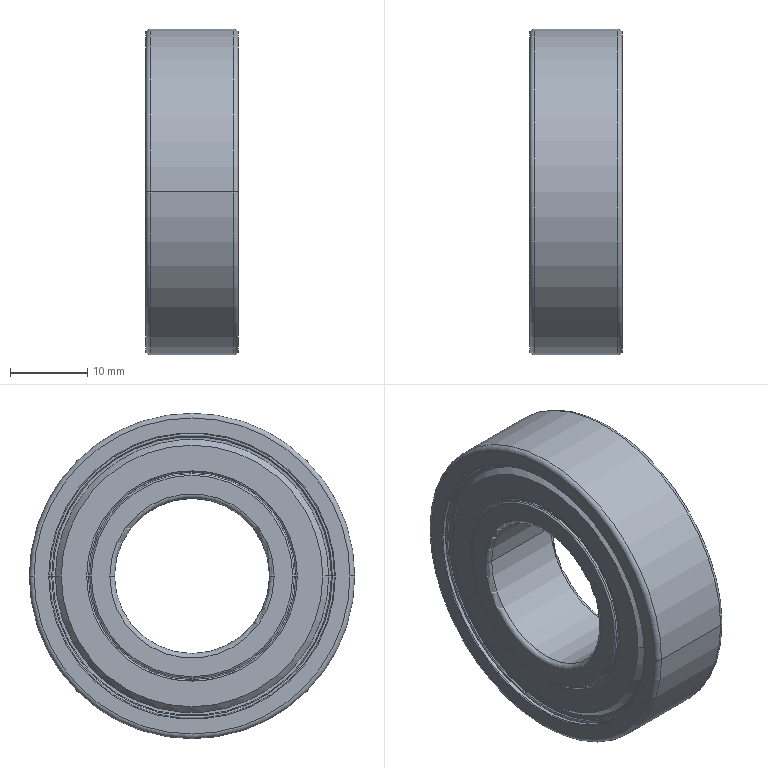Part | STEP file | BAY6004ZZ-bfu61_86-2(2)^BFU71-6004ZZ-L55-S20_Drive roller assembly | 1 solid | 132 faces | box 12 x 42 x 42 mm | volume 10321 mm3 | torus 48 | cone 40 | cylinder 32 | plane 12 | commonest cylinder face diameters 25.6 x4 26.4 x4 26.8 x4 27.2 x4 27.6 x4 35.4 x4